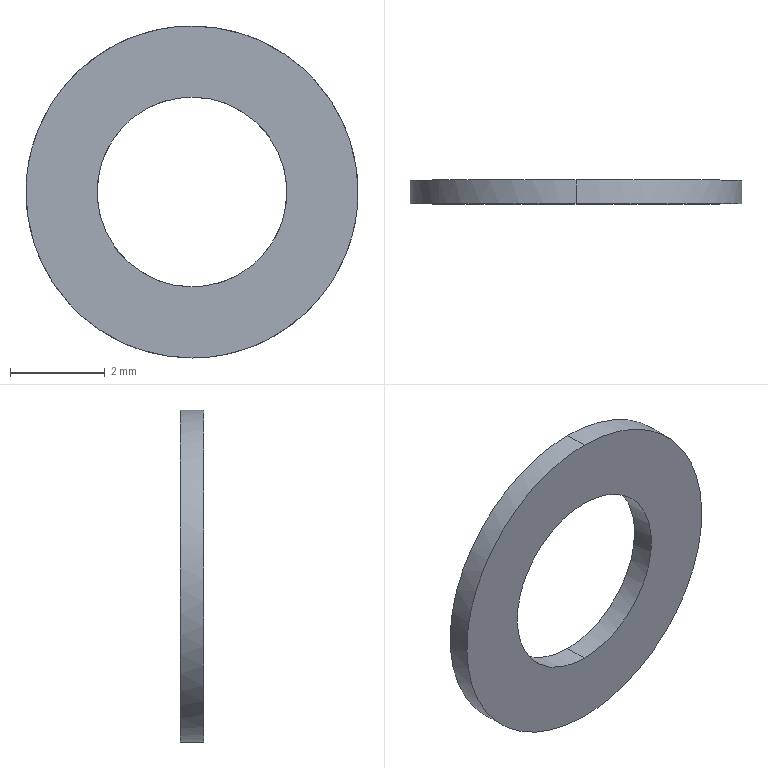Part | SolidWorks | features BaseBody 1 | 1 solid | 6 faces | box 7 x 0.5 x 7 mm | volume 12.959 mm3 | cylinder 4 | plane 2 | commonest cylinder face diameters 4 x2 7 x2
STEP:
#1=CARTESIAN_POINT('',(0.,0.5,3.5));
#2=VERTEX_POINT('',#1);
#3=CARTESIAN_POINT('',(0.,0.5,-3.5));
#4=VERTEX_POINT('',#3);
#5=CARTESIAN_POINT('',(0.,0.5,3.5));
#6=CARTESIAN_POINT('',(0.4641,0.5,3.5));
#7=CARTESIAN_POINT('',(0.9106,0.5,3.411));
#8=CARTESIAN_POINT('',(1.768,0.5,3.056));
#9=CARTESIAN_POINT('',(2.147,0.5,2.803));
#10=CARTESIAN_POINT('',(2.803,0.5,2.147));
#11=CARTESIAN_POINT('',(3.056,0.5,1.768));
#12=CARTESIAN_POINT('',(3.411,0.5,0.9106));
#13=CARTESIAN_POINT('',(3.5,0.5,0.4641));
#14=CARTESIAN_POINT('',(3.5,0.5,-0.4641));
#15=CARTESIAN_POINT('',(3.411,0.5,-0.9106));
#16=CARTESIAN_POINT('',(3.056,0.5,-1.768));
#17=CARTESIAN_POINT('',(2.803,0.5,-2.147));
#18=CARTESIAN_POINT('',(2.147,0.5,-2.803));
#19=CARTESIAN_POINT('',(1.768,0.5,-3.056));
#20=CARTESIAN_POINT('',(0.9106,0.5,-3.411));
#21=CARTESIAN_POINT('',(0.4641,0.5,-3.5));
#22=CARTESIAN_POINT('',(0.,0.5,-3.5));
#23=B_SPLINE_CURVE_WITH_KNOTS('',3,(#5,#6,#7,#8,#9,#10,#11,#12,#13,#14,#15,#16,#17,#18,#19,#20,#21,#22),.UNSPECIFIED.,.F.,.F.,(4,2,2,2,2,2,2,2,4),(4.712,5.105,5.498,5.89,6.283,6.676,7.069,7.461,7.854),.UNSPECIFIED.);
#24=EDGE_CURVE('',#2,#4,#23,.T.);
#25=ORIENTED_EDGE('',*,*,#24,.F.);
#26=CARTESIAN_POINT('',(0.,0.,3.5));
#27=VERTEX_POINT('',#26);
#28=CARTESIAN_POINT('',(0.,0.5,3.5));
#29=DIRECTION('',(0.,-1.,0.));
#30=VECTOR('',#29,1000.);
#31=LINE('',#28,#30);
#32=EDGE_CURVE('',#2,#27,#31,.T.);
#33=ORIENTED_EDGE('',*,*,#32,.T.);
#34=CARTESIAN_POINT('',(0.,0.,-3.5));
#35=VERTEX_POINT('',#34);
#36=CARTESIAN_POINT('',(0.,0.,3.5));
#37=CARTESIAN_POINT('',(0.4581,0.,3.5));
#38=CARTESIAN_POINT('',(0.9161,0.,3.409));
#39=CARTESIAN_POINT('',(1.763,0.,3.058));
#40=CARTESIAN_POINT('',(2.151,0.,2.799));
#41=CARTESIAN_POINT('',(2.799,0.,2.151));
#42=CARTESIAN_POINT('',(3.058,0.,1.763));
#43=CARTESIAN_POINT('',(3.409,0.,0.9161));
#44=CARTESIAN_POINT('',(3.5,0.,0.4581));
#45=CARTESIAN_POINT('',(3.5,0.,-0.4581));
#46=CARTESIAN_POINT('',(3.409,0.,-0.9161));
#47=CARTESIAN_POINT('',(3.058,0.,-1.763));
#48=CARTESIAN_POINT('',(2.799,0.,-2.151));
#49=CARTESIAN_POINT('',(2.151,0.,-2.799));
#50=CARTESIAN_POINT('',(1.763,0.,-3.058));
#51=CARTESIAN_POINT('',(0.9161,0.,-3.409));
#52=CARTESIAN_POINT('',(0.4581,0.,-3.5));
#53=CARTESIAN_POINT('',(0.,0.,-3.5));
#54=B_SPLINE_CURVE_WITH_KNOTS('',3,(#36,#37,#38,#39,#40,#41,#42,#43,#44,#45,#46,#47,#48,#49,#50,#51,#52,#53),.UNSPECIFIED.,.F.,.F.,(4,2,2,2,2,2,2,2,4),(4.712,5.105,5.498,5.89,6.283,6.676,7.069,7.461,7.854),.UNSPECIFIED.);
#55=EDGE_CURVE('',#27,#35,#54,.T.);
#56=ORIENTED_EDGE('',*,*,#55,.T.);
#57=CARTESIAN_POINT('',(0.,0.5,-3.5));
#58=DIRECTION('',(0.,-1.,0.));
#59=VECTOR('',#58,1000.);
#60=LINE('',#57,#59);
#61=EDGE_CURVE('',#4,#35,#60,.T.);
#62=ORIENTED_EDGE('',*,*,#61,.F.);
#63=EDGE_LOOP('',(#25,#33,#56,#62));
#64=FACE_OUTER_BOUND('',#63,.T.);
#65=CARTESIAN_POINT('',(0.,0.5,0.));
#66=DIRECTION('',(0.,-1.,0.));
#67=DIRECTION('',(0.,0.,-1.));
#68=AXIS2_PLACEMENT_3D('',#65,#66,#67);
#69=CYLINDRICAL_SURFACE('',#68,3.5);
#70=ADVANCED_FACE('',(#64),#69,.T.);
#71=CARTESIAN_POINT('',(0.,0.5,-2.));
#72=VERTEX_POINT('',#71);
#73=CARTESIAN_POINT('',(0.,0.5,2.));
#74=VERTEX_POINT('',#73);
#75=CARTESIAN_POINT('',(0.,0.5,-2.));
#76=CARTESIAN_POINT('',(-0.2618,0.5,-2.));
#77=CARTESIAN_POINT('',(-0.5235,0.5,-1.948));
#78=CARTESIAN_POINT('',(-1.007,0.5,-1.748));
#79=CARTESIAN_POINT('',(-1.229,0.5,-1.599));
#80=CARTESIAN_POINT('',(-1.599,0.5,-1.229));
#81=CARTESIAN_POINT('',(-1.748,0.5,-1.007));
#82=CARTESIAN_POINT('',(-1.948,0.5,-0.5235));
#83=CARTESIAN_POINT('',(-2.,0.5,-0.2618));
#84=CARTESIAN_POINT('',(-2.,0.5,0.2618));
#85=CARTESIAN_POINT('',(-1.948,0.5,0.5235));
#86=CARTESIAN_POINT('',(-1.748,0.5,1.007));
#87=CARTESIAN_POINT('',(-1.599,0.5,1.229));
#88=CARTESIAN_POINT('',(-1.229,0.5,1.599));
#89=CARTESIAN_POINT('',(-1.007,0.5,1.748));
#90=CARTESIAN_POINT('',(-0.5235,0.5,1.948));
#91=CARTESIAN_POINT('',(-0.2618,0.5,2.));
#92=CARTESIAN_POINT('',(0.,0.5,2.));
#93=B_SPLINE_CURVE_WITH_KNOTS('',3,(#75,#76,#77,#78,#79,#80,#81,#82,#83,#84,#85,#86,#87,#88,#89,#90,#91,#92),.UNSPECIFIED.,.F.,.F.,(4,2,2,2,2,2,2,2,4),(1.571,1.963,2.356,2.749,3.142,3.534,3.927,4.32,4.712),.UNSPECIFIED.);
#94=EDGE_CURVE('',#72,#74,#93,.T.);
#95=ORIENTED_EDGE('',*,*,#94,.T.);
#96=CARTESIAN_POINT('',(0.,0.,2.));
#97=VERTEX_POINT('',#96);
#98=CARTESIAN_POINT('',(0.,0.5,2.));
#99=DIRECTION('',(0.,-1.,0.));
#100=VECTOR('',#99,1000.);
#101=LINE('',#98,#100);
#102=EDGE_CURVE('',#74,#97,#101,.T.);
#103=ORIENTED_EDGE('',*,*,#102,.T.);
#104=CARTESIAN_POINT('',(0.,0.,-2.));
#105=VERTEX_POINT('',#104);
#106=CARTESIAN_POINT('',(0.,0.,-2.));
#107=CARTESIAN_POINT('',(-0.2652,0.,-2.));
#108=CARTESIAN_POINT('',(-0.5203,0.,-1.949));
#109=CARTESIAN_POINT('',(-1.01,0.,-1.746));
#110=CARTESIAN_POINT('',(-1.227,0.,-1.602));
#111=CARTESIAN_POINT('',(-1.602,0.,-1.227));
#112=CARTESIAN_POINT('',(-1.746,0.,-1.01));
#113=CARTESIAN_POINT('',(-1.949,0.,-0.5203));
#114=CARTESIAN_POINT('',(-2.,0.,-0.2652));
#115=CARTESIAN_POINT('',(-2.,0.,0.2652));
#116=CARTESIAN_POINT('',(-1.949,0.,0.5203));
#117=CARTESIAN_POINT('',(-1.746,0.,1.01));
#118=CARTESIAN_POINT('',(-1.602,0.,1.227));
#119=CARTESIAN_POINT('',(-1.227,0.,1.602));
#120=CARTESIAN_POINT('',(-1.01,0.,1.746));
#121=CARTESIAN_POINT('',(-0.5203,0.,1.949));
#122=CARTESIAN_POINT('',(-0.2652,0.,2.));
#123=CARTESIAN_POINT('',(0.,0.,2.));
#124=B_SPLINE_CURVE_WITH_KNOTS('',3,(#106,#107,#108,#109,#110,#111,#112,#113,#114,#115,#116,#117,#118,#119,#120,#121,#122,#123),.UNSPECIFIED.,.F.,.F.,(4,2,2,2,2,2,2,2,4),(1.571,1.963,2.356,2.749,3.142,3.534,3.927,4.32,4.712),.UNSPECIFIED.);
#125=EDGE_CURVE('',#105,#97,#124,.T.);
#126=ORIENTED_EDGE('',*,*,#125,.F.);
#127=CARTESIAN_POINT('',(0.,0.5,-2.));
#128=DIRECTION('',(0.,-1.,0.));
#129=VECTOR('',#128,1000.);
#130=LINE('',#127,#129);
#131=EDGE_CURVE('',#72,#105,#130,.T.);
#132=ORIENTED_EDGE('',*,*,#131,.F.);
#133=EDGE_LOOP('',(#95,#103,#126,#132));
#134=FACE_OUTER_BOUND('',#133,.T.);
#135=CARTESIAN_POINT('',(0.,0.5,0.));
#136=DIRECTION('',(0.,-1.,0.));
#137=DIRECTION('',(0.,0.,-1.));
#138=AXIS2_PLACEMENT_3D('',#135,#136,#137);
#139=CYLINDRICAL_SURFACE('',#138,2.);
#140=ADVANCED_FACE('',(#134),#139,.F.);
#141=ORIENTED_EDGE('',*,*,#102,.F.);
#142=CARTESIAN_POINT('',(0.,0.5,2.));
#143=CARTESIAN_POINT('',(0.2618,0.5,2.));
#144=CARTESIAN_POINT('',(0.5235,0.5,1.948));
#145=CARTESIAN_POINT('',(1.007,0.5,1.748));
#146=CARTESIAN_POINT('',(1.229,0.5,1.599));
#147=CARTESIAN_POINT('',(1.599,0.5,1.229));
#148=CARTESIAN_POINT('',(1.748,0.5,1.007));
#149=CARTESIAN_POINT('',(1.948,0.5,0.5235));
#150=CARTESIAN_POINT('',(2.,0.5,0.2618));
#151=CARTESIAN_POINT('',(2.,0.5,-0.2618));
#152=CARTESIAN_POINT('',(1.948,0.5,-0.5235));
#153=CARTESIAN_POINT('',(1.748,0.5,-1.007));
#154=CARTESIAN_POINT('',(1.599,0.5,-1.229));
#155=CARTESIAN_POINT('',(1.229,0.5,-1.599));
#156=CARTESIAN_POINT('',(1.007,0.5,-1.748));
#157=CARTESIAN_POINT('',(0.5235,0.5,-1.948));
#158=CARTESIAN_POINT('',(0.2618,0.5,-2.));
#159=CARTESIAN_POINT('',(0.,0.5,-2.));
#160=B_SPLINE_CURVE_WITH_KNOTS('',3,(#142,#143,#144,#145,#146,#147,#148,#149,#150,#151,#152,#153,#154,#155,#156,#157,#158,#159),.UNSPECIFIED.,.F.,.F.,(4,2,2,2,2,2,2,2,4),(4.712,5.105,5.498,5.89,6.283,6.676,7.069,7.461,7.854),.UNSPECIFIED.);
#161=EDGE_CURVE('',#74,#72,#160,.T.);
#162=ORIENTED_EDGE('',*,*,#161,.T.);
#163=ORIENTED_EDGE('',*,*,#131,.T.);
#164=CARTESIAN_POINT('',(0.,0.,2.));
#165=CARTESIAN_POINT('',(0.2652,0.,2.));
#166=CARTESIAN_POINT('',(0.5203,0.,1.949));
#167=CARTESIAN_POINT('',(1.01,0.,1.746));
#168=CARTESIAN_POINT('',(1.227,0.,1.602));
#169=CARTESIAN_POINT('',(1.602,0.,1.227));
#170=CARTESIAN_POINT('',(1.746,0.,1.01));
#171=CARTESIAN_POINT('',(1.949,0.,0.5203));
#172=CARTESIAN_POINT('',(2.,0.,0.2652));
#173=CARTESIAN_POINT('',(2.,0.,-0.2652));
#174=CARTESIAN_POINT('',(1.949,0.,-0.5203));
#175=CARTESIAN_POINT('',(1.746,0.,-1.01));
#176=CARTESIAN_POINT('',(1.602,0.,-1.227));
#177=CARTESIAN_POINT('',(1.227,0.,-1.602));
#178=CARTESIAN_POINT('',(1.01,0.,-1.746));
#179=CARTESIAN_POINT('',(0.5203,0.,-1.949));
#180=CARTESIAN_POINT('',(0.2652,0.,-2.));
#181=CARTESIAN_POINT('',(0.,0.,-2.));
#182=B_SPLINE_CURVE_WITH_KNOTS('',3,(#164,#165,#166,#167,#168,#169,#170,#171,#172,#173,#174,#175,#176,#177,#178,#179,#180,#181),.UNSPECIFIED.,.F.,.F.,(4,2,2,2,2,2,2,2,4),(4.712,5.105,5.498,5.89,6.283,6.676,7.069,7.461,7.854),.UNSPECIFIED.);
#183=EDGE_CURVE('',#97,#105,#182,.T.);
#184=ORIENTED_EDGE('',*,*,#183,.F.);
#185=EDGE_LOOP('',(#141,#162,#163,#184));
#186=FACE_OUTER_BOUND('',#185,.T.);
#187=CARTESIAN_POINT('',(0.,0.5,0.));
#188=DIRECTION('',(0.,-1.,0.));
#189=DIRECTION('',(0.,0.,-1.));
#190=AXIS2_PLACEMENT_3D('',#187,#188,#189);
#191=CYLINDRICAL_SURFACE('',#190,2.);
#192=ADVANCED_FACE('',(#186),#191,.F.);
#193=ORIENTED_EDGE('',*,*,#32,.F.);
#194=CARTESIAN_POINT('',(0.,0.5,-3.5));
#195=CARTESIAN_POINT('',(-0.4641,0.5,-3.5));
#196=CARTESIAN_POINT('',(-0.9106,0.5,-3.411));
#197=CARTESIAN_POINT('',(-1.768,0.5,-3.056));
#198=CARTESIAN_POINT('',(-2.147,0.5,-2.803));
#199=CARTESIAN_POINT('',(-2.803,0.5,-2.147));
#200=CARTESIAN_POINT('',(-3.056,0.5,-1.768));
#201=CARTESIAN_POINT('',(-3.411,0.5,-0.9106));
#202=CARTESIAN_POINT('',(-3.5,0.5,-0.4641));
#203=CARTESIAN_POINT('',(-3.5,0.5,0.4641));
#204=CARTESIAN_POINT('',(-3.411,0.5,0.9106));
#205=CARTESIAN_POINT('',(-3.056,0.5,1.768));
#206=CARTESIAN_POINT('',(-2.803,0.5,2.147));
#207=CARTESIAN_POINT('',(-2.147,0.5,2.803));
#208=CARTESIAN_POINT('',(-1.768,0.5,3.056));
#209=CARTESIAN_POINT('',(-0.9106,0.5,3.411));
#210=CARTESIAN_POINT('',(-0.4641,0.5,3.5));
#211=CARTESIAN_POINT('',(0.,0.5,3.5));
#212=B_SPLINE_CURVE_WITH_KNOTS('',3,(#194,#195,#196,#197,#198,#199,#200,#201,#202,#203,#204,#205,#206,#207,#208,#209,#210,#211),.UNSPECIFIED.,.F.,.F.,(4,2,2,2,2,2,2,2,4),(1.571,1.963,2.356,2.749,3.142,3.534,3.927,4.32,4.712),.UNSPECIFIED.);
#213=EDGE_CURVE('',#4,#2,#212,.T.);
#214=ORIENTED_EDGE('',*,*,#213,.F.);
#215=ORIENTED_EDGE('',*,*,#61,.T.);
#216=CARTESIAN_POINT('',(0.,0.,-3.5));
#217=CARTESIAN_POINT('',(-0.4581,0.,-3.5));
#218=CARTESIAN_POINT('',(-0.9161,0.,-3.409));
#219=CARTESIAN_POINT('',(-1.763,0.,-3.058));
#220=CARTESIAN_POINT('',(-2.151,0.,-2.799));
#221=CARTESIAN_POINT('',(-2.799,0.,-2.151));
#222=CARTESIAN_POINT('',(-3.058,0.,-1.763));
#223=CARTESIAN_POINT('',(-3.409,0.,-0.9161));
#224=CARTESIAN_POINT('',(-3.5,0.,-0.4581));
#225=CARTESIAN_POINT('',(-3.5,0.,0.4581));
#226=CARTESIAN_POINT('',(-3.409,0.,0.9161));
#227=CARTESIAN_POINT('',(-3.058,0.,1.763));
#228=CARTESIAN_POINT('',(-2.799,0.,2.151));
#229=CARTESIAN_POINT('',(-2.151,0.,2.799));
#230=CARTESIAN_POINT('',(-1.763,0.,3.058));
#231=CARTESIAN_POINT('',(-0.9161,0.,3.409));
#232=CARTESIAN_POINT('',(-0.4581,0.,3.5));
#233=CARTESIAN_POINT('',(0.,0.,3.5));
#234=B_SPLINE_CURVE_WITH_KNOTS('',3,(#216,#217,#218,#219,#220,#221,#222,#223,#224,#225,#226,#227,#228,#229,#230,#231,#232,#233),.UNSPECIFIED.,.F.,.F.,(4,2,2,2,2,2,2,2,4),(1.571,1.963,2.356,2.749,3.142,3.534,3.927,4.32,4.712),.UNSPECIFIED.);
#235=EDGE_CURVE('',#35,#27,#234,.T.);
#236=ORIENTED_EDGE('',*,*,#235,.T.);
#237=EDGE_LOOP('',(#193,#214,#215,#236));
#238=FACE_OUTER_BOUND('',#237,.T.);
#239=CARTESIAN_POINT('',(0.,0.5,0.));
#240=DIRECTION('',(0.,-1.,0.));
#241=DIRECTION('',(0.,0.,-1.));
#242=AXIS2_PLACEMENT_3D('',#239,#240,#241);
#243=CYLINDRICAL_SURFACE('',#242,3.5);
#244=ADVANCED_FACE('',(#238),#243,.T.);
#245=ORIENTED_EDGE('',*,*,#94,.F.);
#246=ORIENTED_EDGE('',*,*,#161,.F.);
#247=EDGE_LOOP('',(#245,#246));
#248=FACE_BOUND('',#247,.T.);
#249=ORIENTED_EDGE('',*,*,#213,.T.);
#250=ORIENTED_EDGE('',*,*,#24,.T.);
#251=EDGE_LOOP('',(#249,#250));
#252=FACE_OUTER_BOUND('',#251,.T.);
#253=CARTESIAN_POINT('',(0.,0.5,0.));
#254=DIRECTION('',(0.,1.,0.));
#255=DIRECTION('',(0.,0.,1.));
#256=AXIS2_PLACEMENT_3D('',#253,#254,#255);
#257=PLANE('',#256);
#258=ADVANCED_FACE('',(#248,#252),#257,.T.);
#259=ORIENTED_EDGE('',*,*,#125,.T.);
#260=ORIENTED_EDGE('',*,*,#183,.T.);
#261=EDGE_LOOP('',(#259,#260));
#262=FACE_BOUND('',#261,.T.);
#263=ORIENTED_EDGE('',*,*,#235,.F.);
#264=ORIENTED_EDGE('',*,*,#55,.F.);
#265=EDGE_LOOP('',(#263,#264));
#266=FACE_OUTER_BOUND('',#265,.T.);
#267=CARTESIAN_POINT('',(0.,0.,0.));
#268=DIRECTION('',(0.,1.,0.));
#269=DIRECTION('',(0.,0.,1.));
#270=AXIS2_PLACEMENT_3D('',#267,#268,#269);
#271=PLANE('',#270);
#272=ADVANCED_FACE('',(#262,#266),#271,.F.);
#273=CLOSED_SHELL('',(#70,#140,#192,#244,#258,#272));
#274=MANIFOLD_SOLID_BREP('',#273);
#275=CARTESIAN_POINT('',(0.,0.,0.));
#276=DIRECTION('',(0.,0.,1.));
#277=DIRECTION('',(1.,0.,0.));
#278=AXIS2_PLACEMENT_3D('',#275,#276,#277);
#279=(LENGTH_UNIT()NAMED_UNIT(*)SI_UNIT(.MILLI.,.METRE.));
#280=UNCERTAINTY_MEASURE_WITH_UNIT(LENGTH_MEASURE(0.00001),#279,'','');
#281=(NAMED_UNIT(*)PLANE_ANGLE_UNIT()SI_UNIT($,.RADIAN.));
#282=(NAMED_UNIT(*)SI_UNIT($,.STERADIAN.)SOLID_ANGLE_UNIT());
#283=(GEOMETRIC_REPRESENTATION_CONTEXT(3)GLOBAL_UNCERTAINTY_ASSIGNED_CONTEXT((#280))GLOBAL_UNIT_ASSIGNED_CONTEXT((#279,#281,#282))REPRESENTATION_CONTEXT('',''));
#284=ADVANCED_BREP_SHAPE_REPRESENTATION('',(#274,#278),#283);